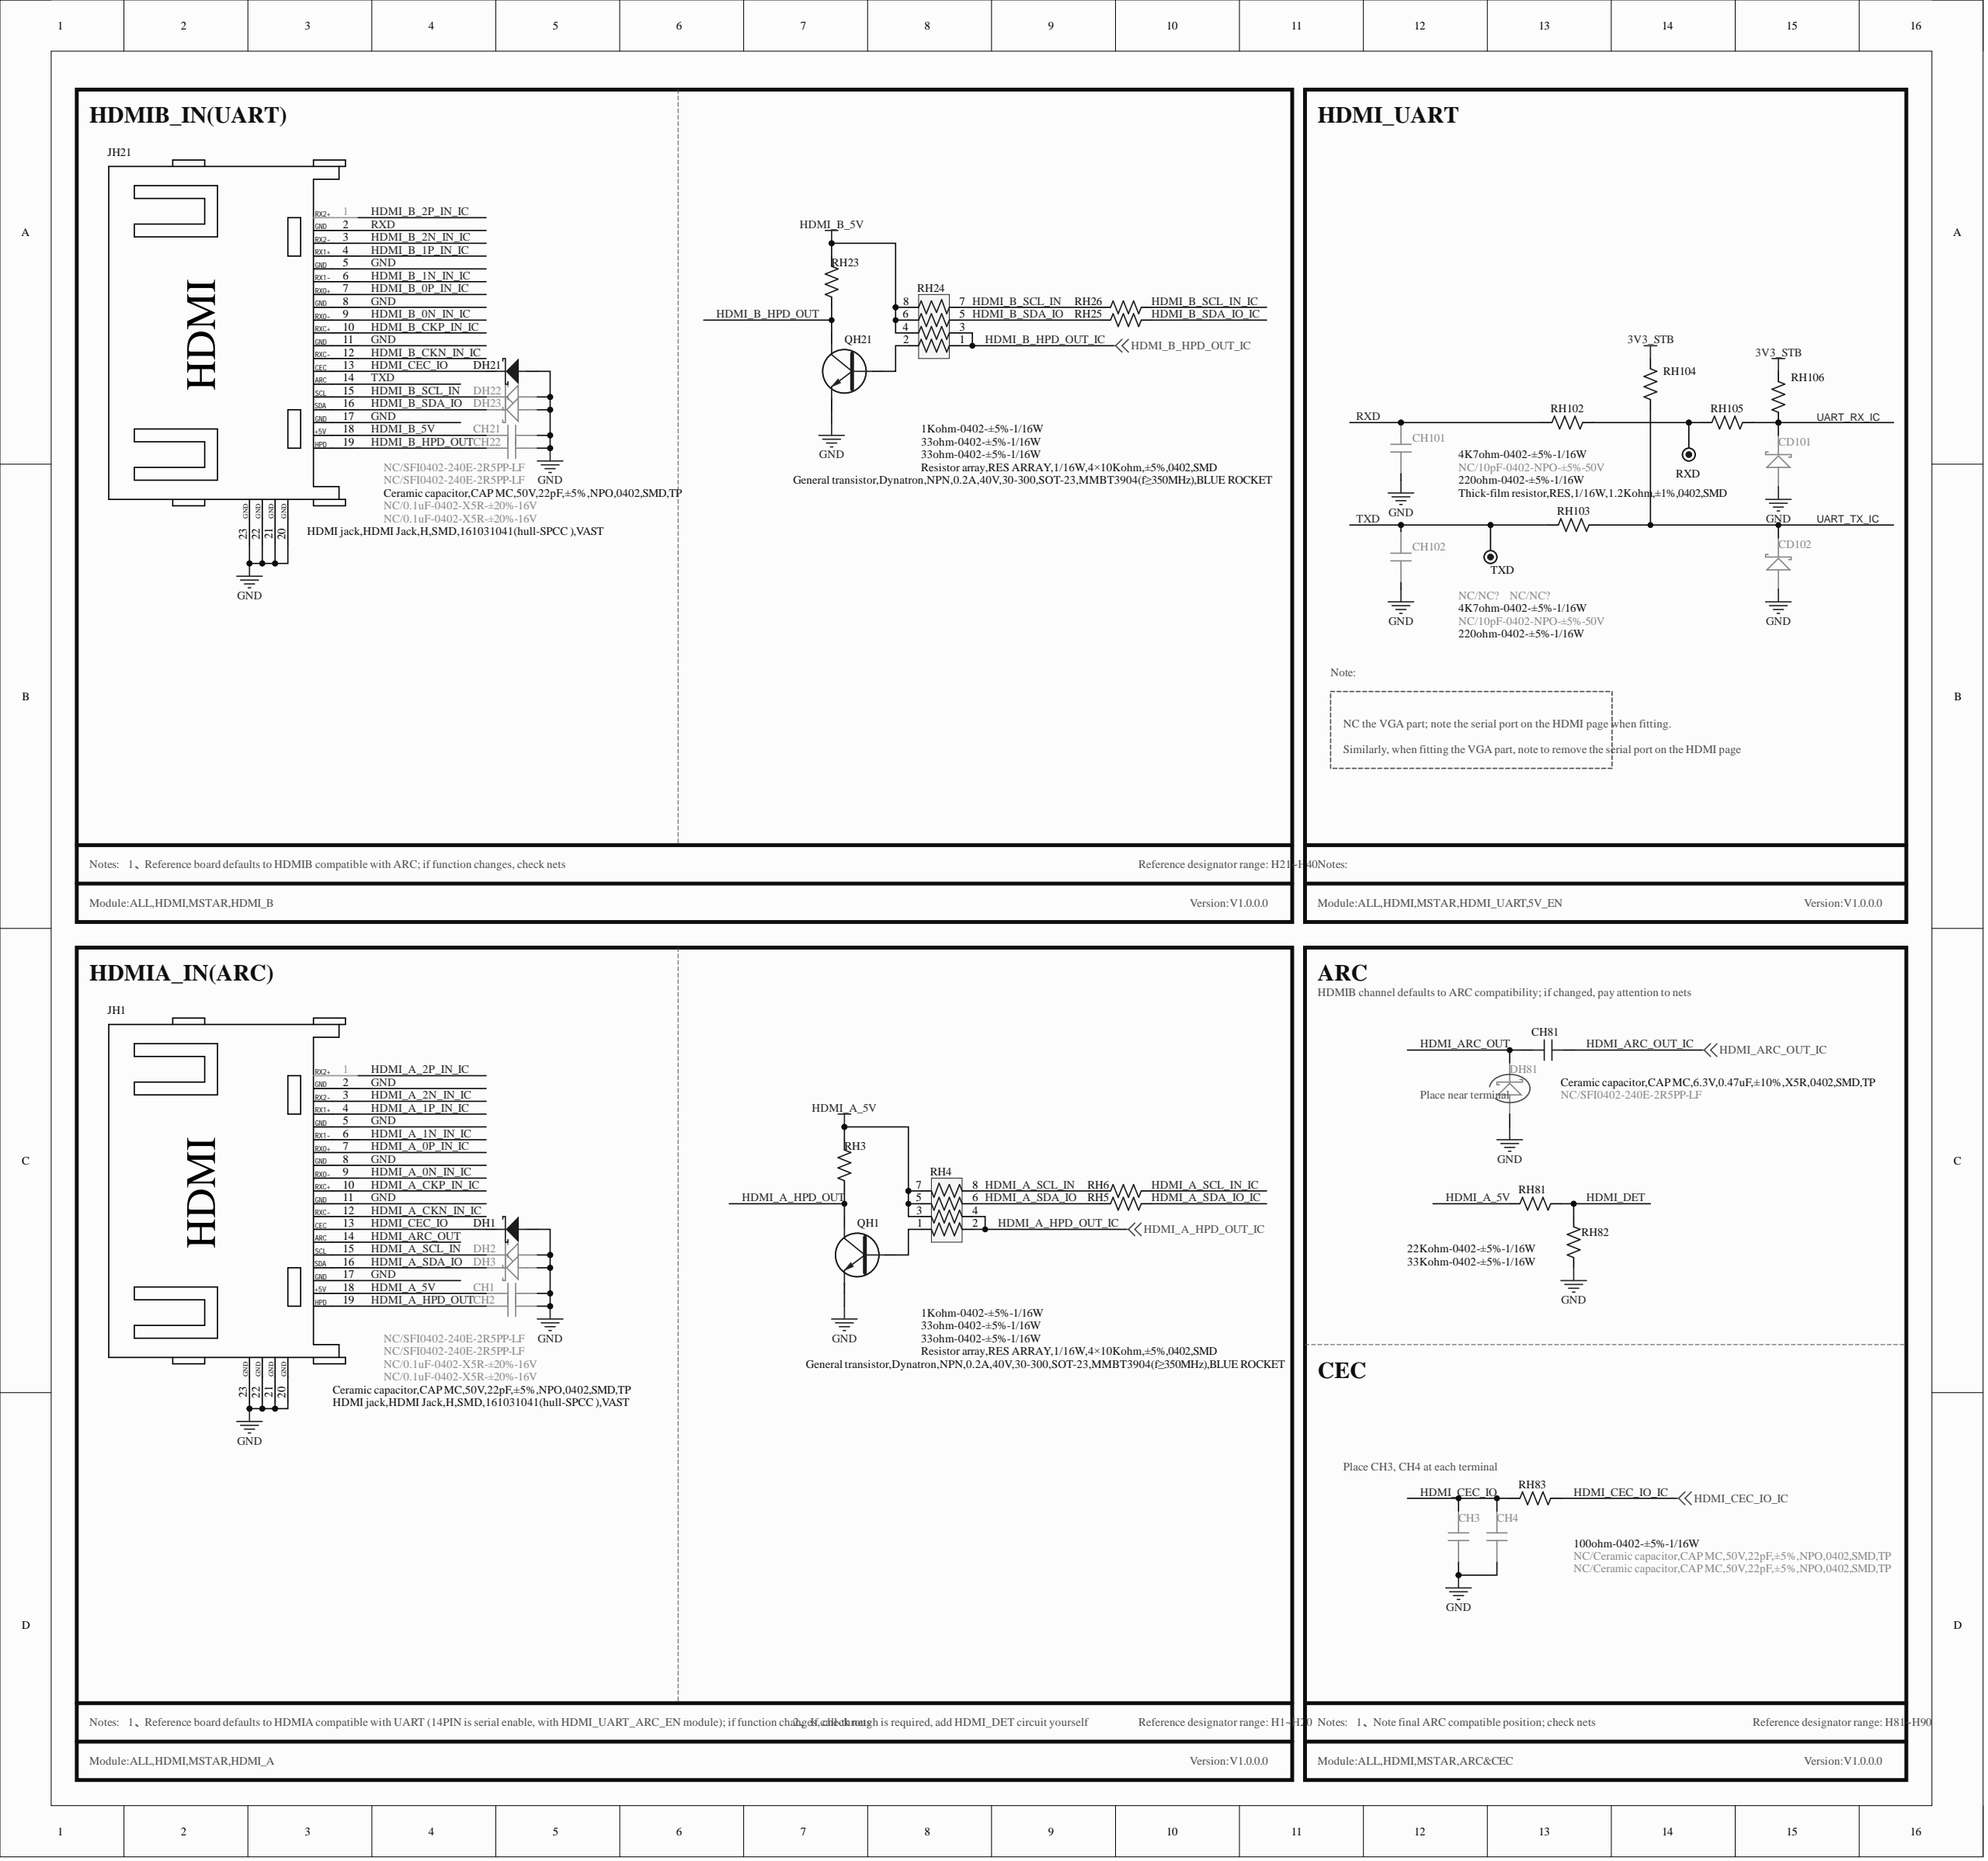Circuit board | Altium Designer | 578 parts | 300 nets | one sheet of the schematic
Parts on this sheet (reference | value | footprint):
CD101 | NC/NC? | DIODE-S0402
CD102 | NC/NC? | DIODE-S0402
CH1 | NC/0.1uF-0402-X5R-±20%-16V | C0402
CH2 | NC/0.1uF-0402-X5R-±20%-16V | C0402
CH3 | NC/Ceramic capacitor,CAP MC,50V,22pF,±5%,NPO,0402,SMD,TP | C0402
CH4 | NC/Ceramic capacitor,CAP MC,50V,22pF,±5%,NPO,0402,SMD,TP | C0402
CH21 | NC/0.1uF-0402-X5R-±20%-16V | C0402
CH22 | NC/0.1uF-0402-X5R-±20%-16V | C0402
CH81 | Ceramic capacitor,CAP MC,6.3V,0.47uF,±10%,X5R,0402,SMD,TP | C0402
CH101 | NC/10pF-0402-NPO-±5%-50V | C0402
CH102 | NC/10pF-0402-NPO-±5%-50V | C0402
DH1 | Ceramic capacitor,CAP MC,50V,22pF,±5%,NPO,0402,SMD,TP | DIODE-S0402
DH2 | NC/SFI0402-240E-2R5PP-LF | DIODE-S0402
DH3 | NC/SFI0402-240E-2R5PP-LF | DIODE-S0402
DH21 | Ceramic capacitor,CAP MC,50V,22pF,±5%,NPO,0402,SMD,TP | DIODE-S0402
DH22 | NC/SFI0402-240E-2R5PP-LF | DIODE-S0402
DH23 | NC/SFI0402-240E-2R5PP-LF | DIODE-S0402
DH81 | NC/SFI0402-240E-2R5PP-LF | DIODE-S0402
JH1 | HDMI jack,HDMI Jack,H,SMD,161031041(hull-SPCC ),VAST | HDMI-HS-1
JH21 | HDMI jack,HDMI Jack,H,SMD,161031041(hull-SPCC ),VAST | HDMI-HS-1
QH1 | General transistor,Dynatron,NPN,0.2A,40V,30-300,SOT-23,MMBT3904(f=350MHz),BLUE ROCKET | SOT-23
QH21 | General transistor,Dynatron,NPN,0.2A,40V,30-300,SOT-23,MMBT3904(f=350MHz),BLUE ROCKET | SOT-23
RH3 | 1Kohm-0402-±5%-1/16W | R0402
RH4 | Resistor array,RES ARRAY,1/16W,4×10Kohm,±5%,0402,SMD | RA0402
RH5 | 33ohm-0402-±5%-1/16W | R0402
RH6 | 33ohm-0402-±5%-1/16W | R0402
RH23 | 1Kohm-0402-±5%-1/16W | R0402
RH24 | Resistor array,RES ARRAY,1/16W,4×10Kohm,±5%,0402,SMD | RA0402
RH25 | 33ohm-0402-±5%-1/16W | R0402
RH26 | 33ohm-0402-±5%-1/16W | R0402
RH81 | 22Kohm-0402-±5%-1/16W | R0402
RH82 | 33Kohm-0402-±5%-1/16W | R0402
RH83 | 100ohm-0402-±5%-1/16W | R0402
RH102 | Thick-film resistor,RES,1/16W,1.2Kohm,±1%,0402,SMD | R0402
RH103 | 220ohm-0402-±5%-1/16W | R0402
RH104 | 4K7ohm-0402-±5%-1/16W | R0402
RH105 | 220ohm-0402-±5%-1/16W | R0402
RH106 | 4K7ohm-0402-±5%-1/16W | R0402
Nets of these parts (net: part-pin ...):
UART_TX_IC: CD102-K RH103-2 RH104-1
UART_RX_IC: CD101-K RH105-2 RH106-1
TXD: CH102-2 RH103-1 JH21-14
RXD: CH101-2 RH102-1 JH21-2
NetRH102_2: RH102-2 RH105-1
NetQH21_B: QH21-B RH24-2
NetQH1_B: QH1-B RH4-1
HDMI_DET: RH81-1 RH82-1
HDMI_CEC_IO_IC: RH83-1
HDMI_CEC_IO: CH3-2 CH4-2 DH1-K DH21-K RH83-2 JH1-13 JH21-13
HDMI_B_SDA_IO_IC: RH25-2
HDMI_B_SDA_IO: DH23-K RH24-5 RH25-1 JH21-16
HDMI_B_SCL_IN_IC: RH26-2
HDMI_B_SCL_IN: DH22-K RH24-7 RH26-1 JH21-15
HDMI_B_HPD_OUT_IC: RH24-1 RH24-3
HDMI_B_HPD_OUT: CH22-1 QH21-C RH23-1 JH21-19
HDMI_B_CKP_IN_IC: JH21-10
HDMI_B_CKN_IN_IC: JH21-12
HDMI_B_5V: CH21-1 RH23-2 RH24-4 RH24-6 RH24-8 JH21-18
HDMI_B_2P_IN_IC: JH21-1
HDMI_B_2N_IN_IC: JH21-3
HDMI_B_1P_IN_IC: JH21-4
HDMI_B_1N_IN_IC: JH21-6
HDMI_B_0P_IN_IC: JH21-7
HDMI_B_0N_IN_IC: JH21-9
HDMI_ARC_OUT_IC: CH81-2
HDMI_ARC_OUT: CH81-1 DH81-K JH1-14
HDMI_A_SDA_IO_IC: RH5-2
HDMI_A_SDA_IO: DH3-K RH4-6 RH5-1 JH1-16
HDMI_A_SCL_IN_IC: RH6-2
HDMI_A_SCL_IN: DH2-K RH4-8 RH6-1 JH1-15
HDMI_A_HPD_OUT_IC: RH4-2 RH4-4
HDMI_A_HPD_OUT: CH2-1 QH1-C RH3-1 JH1-19
HDMI_A_CKP_IN_IC: JH1-10
HDMI_A_CKN_IN_IC: JH1-12
HDMI_A_5V: CH1-1 RH3-2 RH4-3 RH4-5 RH4-7 RH81-2 JH1-18
HDMI_A_2P_IN_IC: JH1-1
HDMI_A_2N_IN_IC: JH1-3
HDMI_A_1P_IN_IC: JH1-4
HDMI_A_1N_IN_IC: JH1-6
HDMI_A_0P_IN_IC: JH1-7
HDMI_A_0N_IN_IC: JH1-9
GND: CD101-A CD102-A CH1-2 CH2-2 CH3-1 CH4-1 CH21-2 CH22-2 CH101-1 CH102-1 DH1-A DH2-A DH3-A DH21-A DH22-A DH23-A DH81-A QH1-E QH21-E RH82-2 JH1-2 JH1-5 JH1-8 JH1-11 JH1-17 JH1-20 JH1-21 JH1-22 JH1-23 JH21-5 JH21-8 JH21-11 JH21-17 JH21-20 JH21-21 JH21-22 JH21-23
3V3_STB: RH104-2 RH106-2